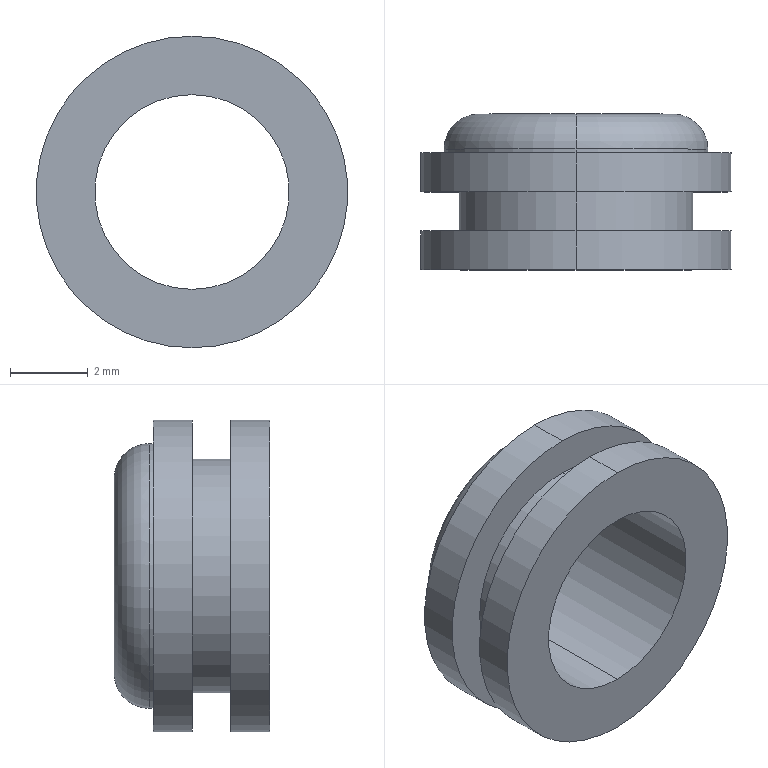Part | SolidWorks | features Revolution 1 | 1 solid | 16 faces | box 8 x 4 x 8 mm | volume 83.088 mm3 | cylinder 10 | plane 4 | torus 2 | commonest cylinder face diameters 8 x4 5 x2 6 x2 6.8 x2
STEP:
#1=CARTESIAN_POINT('',(0.,3.1,-3.4));
#2=VERTEX_POINT('',#1);
#3=CARTESIAN_POINT('',(0.,3.1,3.4));
#4=VERTEX_POINT('',#3);
#5=CARTESIAN_POINT('',(0.,3.1,0.));
#6=DIRECTION('',(0.,-1.,0.));
#7=DIRECTION('',(0.,0.,-1.));
#8=AXIS2_PLACEMENT_3D('',#5,#6,#7);
#9=CIRCLE('',#8,3.4);
#10=EDGE_CURVE('',#2,#4,#9,.T.);
#11=ORIENTED_EDGE('',*,*,#10,.T.);
#12=CARTESIAN_POINT('',(0.,3.,3.4));
#13=VERTEX_POINT('',#12);
#14=CARTESIAN_POINT('',(0.,0.,3.4));
#15=DIRECTION('',(0.,-1.,0.));
#16=VECTOR('',#15,1000.);
#17=LINE('',#14,#16);
#18=EDGE_CURVE('',#4,#13,#17,.T.);
#19=ORIENTED_EDGE('',*,*,#18,.T.);
#20=CARTESIAN_POINT('',(0.,3.,-3.4));
#21=VERTEX_POINT('',#20);
#22=CARTESIAN_POINT('',(0.,3.,0.));
#23=DIRECTION('',(0.,-1.,0.));
#24=DIRECTION('',(0.,0.,-1.));
#25=AXIS2_PLACEMENT_3D('',#22,#23,#24);
#26=CIRCLE('',#25,3.4);
#27=EDGE_CURVE('',#21,#13,#26,.T.);
#28=ORIENTED_EDGE('',*,*,#27,.F.);
#29=CARTESIAN_POINT('',(0.,0.,-3.4));
#30=DIRECTION('',(0.,-1.,0.));
#31=VECTOR('',#30,1000.);
#32=LINE('',#29,#31);
#33=EDGE_CURVE('',#2,#21,#32,.T.);
#34=ORIENTED_EDGE('',*,*,#33,.F.);
#35=EDGE_LOOP('',(#11,#19,#28,#34));
#36=FACE_OUTER_BOUND('',#35,.T.);
#37=CARTESIAN_POINT('',(0.,0.,0.));
#38=DIRECTION('',(0.,-1.,0.));
#39=DIRECTION('',(0.,0.,-1.));
#40=AXIS2_PLACEMENT_3D('',#37,#38,#39);
#41=CYLINDRICAL_SURFACE('',#40,3.4);
#42=ADVANCED_FACE('',(#36),#41,.T.);
#43=CARTESIAN_POINT('',(0.,3.,-4.));
#44=VERTEX_POINT('',#43);
#45=CARTESIAN_POINT('',(0.,3.,4.));
#46=VERTEX_POINT('',#45);
#47=CARTESIAN_POINT('',(0.,3.,0.));
#48=DIRECTION('',(0.,-1.,0.));
#49=DIRECTION('',(0.,0.,-1.));
#50=AXIS2_PLACEMENT_3D('',#47,#48,#49);
#51=CIRCLE('',#50,4.);
#52=EDGE_CURVE('',#44,#46,#51,.T.);
#53=ORIENTED_EDGE('',*,*,#52,.T.);
#54=CARTESIAN_POINT('',(0.,2.,4.));
#55=VERTEX_POINT('',#54);
#56=CARTESIAN_POINT('',(0.,0.,4.));
#57=DIRECTION('',(0.,-1.,0.));
#58=VECTOR('',#57,1000.);
#59=LINE('',#56,#58);
#60=EDGE_CURVE('',#46,#55,#59,.T.);
#61=ORIENTED_EDGE('',*,*,#60,.T.);
#62=CARTESIAN_POINT('',(0.,2.,-4.));
#63=VERTEX_POINT('',#62);
#64=CARTESIAN_POINT('',(0.,2.,0.));
#65=DIRECTION('',(0.,-1.,0.));
#66=DIRECTION('',(0.,0.,-1.));
#67=AXIS2_PLACEMENT_3D('',#64,#65,#66);
#68=CIRCLE('',#67,4.);
#69=EDGE_CURVE('',#63,#55,#68,.T.);
#70=ORIENTED_EDGE('',*,*,#69,.F.);
#71=CARTESIAN_POINT('',(0.,0.,-4.));
#72=DIRECTION('',(0.,-1.,0.));
#73=VECTOR('',#72,1000.);
#74=LINE('',#71,#73);
#75=EDGE_CURVE('',#44,#63,#74,.T.);
#76=ORIENTED_EDGE('',*,*,#75,.F.);
#77=EDGE_LOOP('',(#53,#61,#70,#76));
#78=FACE_OUTER_BOUND('',#77,.T.);
#79=CARTESIAN_POINT('',(0.,0.,0.));
#80=DIRECTION('',(0.,-1.,0.));
#81=DIRECTION('',(0.,0.,-1.));
#82=AXIS2_PLACEMENT_3D('',#79,#80,#81);
#83=CYLINDRICAL_SURFACE('',#82,4.);
#84=ADVANCED_FACE('',(#78),#83,.T.);
#85=CARTESIAN_POINT('',(0.,2.,-3.));
#86=VERTEX_POINT('',#85);
#87=CARTESIAN_POINT('',(0.,2.,3.));
#88=VERTEX_POINT('',#87);
#89=CARTESIAN_POINT('',(0.,2.,0.));
#90=DIRECTION('',(0.,-1.,0.));
#91=DIRECTION('',(0.,0.,-1.));
#92=AXIS2_PLACEMENT_3D('',#89,#90,#91);
#93=CIRCLE('',#92,3.);
#94=EDGE_CURVE('',#86,#88,#93,.T.);
#95=ORIENTED_EDGE('',*,*,#94,.T.);
#96=CARTESIAN_POINT('',(0.,1.,3.));
#97=VERTEX_POINT('',#96);
#98=CARTESIAN_POINT('',(0.,0.,3.));
#99=DIRECTION('',(0.,-1.,0.));
#100=VECTOR('',#99,1000.);
#101=LINE('',#98,#100);
#102=EDGE_CURVE('',#88,#97,#101,.T.);
#103=ORIENTED_EDGE('',*,*,#102,.T.);
#104=CARTESIAN_POINT('',(0.,1.,-3.));
#105=VERTEX_POINT('',#104);
#106=CARTESIAN_POINT('',(0.,1.,0.));
#107=DIRECTION('',(0.,-1.,0.));
#108=DIRECTION('',(0.,0.,-1.));
#109=AXIS2_PLACEMENT_3D('',#106,#107,#108);
#110=CIRCLE('',#109,3.);
#111=EDGE_CURVE('',#105,#97,#110,.T.);
#112=ORIENTED_EDGE('',*,*,#111,.F.);
#113=CARTESIAN_POINT('',(0.,0.,-3.));
#114=DIRECTION('',(0.,-1.,0.));
#115=VECTOR('',#114,1000.);
#116=LINE('',#113,#115);
#117=EDGE_CURVE('',#86,#105,#116,.T.);
#118=ORIENTED_EDGE('',*,*,#117,.F.);
#119=EDGE_LOOP('',(#95,#103,#112,#118));
#120=FACE_OUTER_BOUND('',#119,.T.);
#121=CARTESIAN_POINT('',(0.,0.,0.));
#122=DIRECTION('',(0.,-1.,0.));
#123=DIRECTION('',(0.,0.,-1.));
#124=AXIS2_PLACEMENT_3D('',#121,#122,#123);
#125=CYLINDRICAL_SURFACE('',#124,3.);
#126=ADVANCED_FACE('',(#120),#125,.T.);
#127=CARTESIAN_POINT('',(0.,1.,-4.));
#128=VERTEX_POINT('',#127);
#129=CARTESIAN_POINT('',(0.,1.,4.));
#130=VERTEX_POINT('',#129);
#131=CARTESIAN_POINT('',(0.,1.,0.));
#132=DIRECTION('',(0.,-1.,0.));
#133=DIRECTION('',(0.,0.,-1.));
#134=AXIS2_PLACEMENT_3D('',#131,#132,#133);
#135=CIRCLE('',#134,4.);
#136=EDGE_CURVE('',#128,#130,#135,.T.);
#137=ORIENTED_EDGE('',*,*,#136,.T.);
#138=CARTESIAN_POINT('',(0.,0.,4.));
#139=VERTEX_POINT('',#138);
#140=CARTESIAN_POINT('',(0.,0.,4.));
#141=DIRECTION('',(0.,-1.,0.));
#142=VECTOR('',#141,1000.);
#143=LINE('',#140,#142);
#144=EDGE_CURVE('',#130,#139,#143,.T.);
#145=ORIENTED_EDGE('',*,*,#144,.T.);
#146=CARTESIAN_POINT('',(0.,0.,-4.));
#147=VERTEX_POINT('',#146);
#148=CARTESIAN_POINT('',(0.,0.,0.));
#149=DIRECTION('',(0.,-1.,0.));
#150=DIRECTION('',(0.,0.,-1.));
#151=AXIS2_PLACEMENT_3D('',#148,#149,#150);
#152=CIRCLE('',#151,4.);
#153=EDGE_CURVE('',#147,#139,#152,.T.);
#154=ORIENTED_EDGE('',*,*,#153,.F.);
#155=CARTESIAN_POINT('',(0.,0.,-4.));
#156=DIRECTION('',(0.,-1.,0.));
#157=VECTOR('',#156,1000.);
#158=LINE('',#155,#157);
#159=EDGE_CURVE('',#128,#147,#158,.T.);
#160=ORIENTED_EDGE('',*,*,#159,.F.);
#161=EDGE_LOOP('',(#137,#145,#154,#160));
#162=FACE_OUTER_BOUND('',#161,.T.);
#163=CARTESIAN_POINT('',(0.,0.,0.));
#164=DIRECTION('',(0.,-1.,0.));
#165=DIRECTION('',(0.,0.,-1.));
#166=AXIS2_PLACEMENT_3D('',#163,#164,#165);
#167=CYLINDRICAL_SURFACE('',#166,4.);
#168=ADVANCED_FACE('',(#162),#167,.T.);
#169=CARTESIAN_POINT('',(0.,4.,2.5));
#170=VERTEX_POINT('',#169);
#171=CARTESIAN_POINT('',(0.,4.,-2.5));
#172=VERTEX_POINT('',#171);
#173=CARTESIAN_POINT('',(0.,4.,0.));
#174=DIRECTION('',(0.,-1.,0.));
#175=DIRECTION('',(0.,0.,-1.));
#176=AXIS2_PLACEMENT_3D('',#173,#174,#175);
#177=CIRCLE('',#176,2.5);
#178=EDGE_CURVE('',#170,#172,#177,.T.);
#179=ORIENTED_EDGE('',*,*,#178,.F.);
#180=CARTESIAN_POINT('',(0.,0.,2.5));
#181=VERTEX_POINT('',#180);
#182=CARTESIAN_POINT('',(0.,0.,2.5));
#183=DIRECTION('',(0.,-1.,0.));
#184=VECTOR('',#183,1000.);
#185=LINE('',#182,#184);
#186=EDGE_CURVE('',#170,#181,#185,.T.);
#187=ORIENTED_EDGE('',*,*,#186,.T.);
#188=CARTESIAN_POINT('',(0.,0.,-2.5));
#189=VERTEX_POINT('',#188);
#190=CARTESIAN_POINT('',(0.,0.,0.));
#191=DIRECTION('',(0.,-1.,0.));
#192=DIRECTION('',(0.,0.,-1.));
#193=AXIS2_PLACEMENT_3D('',#190,#191,#192);
#194=CIRCLE('',#193,2.5);
#195=EDGE_CURVE('',#181,#189,#194,.T.);
#196=ORIENTED_EDGE('',*,*,#195,.T.);
#197=CARTESIAN_POINT('',(0.,0.,-2.5));
#198=DIRECTION('',(0.,-1.,0.));
#199=VECTOR('',#198,1000.);
#200=LINE('',#197,#199);
#201=EDGE_CURVE('',#172,#189,#200,.T.);
#202=ORIENTED_EDGE('',*,*,#201,.F.);
#203=EDGE_LOOP('',(#179,#187,#196,#202));
#204=FACE_OUTER_BOUND('',#203,.T.);
#205=CARTESIAN_POINT('',(0.,0.,0.));
#206=DIRECTION('',(0.,-1.,0.));
#207=DIRECTION('',(0.,0.,-1.));
#208=AXIS2_PLACEMENT_3D('',#205,#206,#207);
#209=CYLINDRICAL_SURFACE('',#208,2.5);
#210=ADVANCED_FACE('',(#204),#209,.F.);
#211=CARTESIAN_POINT('',(0.,4.,0.));
#212=DIRECTION('',(0.,-1.,0.));
#213=DIRECTION('',(0.,0.,-1.));
#214=AXIS2_PLACEMENT_3D('',#211,#212,#213);
#215=CIRCLE('',#214,2.5);
#216=EDGE_CURVE('',#172,#170,#215,.T.);
#217=ORIENTED_EDGE('',*,*,#216,.T.);
#218=CARTESIAN_POINT('',(0.,3.1,2.5));
#219=DIRECTION('',(1.,0.,0.));
#220=DIRECTION('',(0.,0.,-1.));
#221=AXIS2_PLACEMENT_3D('',#218,#219,#220);
#222=CIRCLE('',#221,0.9);
#223=EDGE_CURVE('',#170,#4,#222,.T.);
#224=ORIENTED_EDGE('',*,*,#223,.T.);
#225=ORIENTED_EDGE('',*,*,#10,.F.);
#226=CARTESIAN_POINT('',(0.,3.1,-2.5));
#227=DIRECTION('',(-1.,0.,0.));
#228=DIRECTION('',(0.,0.,1.));
#229=AXIS2_PLACEMENT_3D('',#226,#227,#228);
#230=CIRCLE('',#229,0.9);
#231=EDGE_CURVE('',#172,#2,#230,.T.);
#232=ORIENTED_EDGE('',*,*,#231,.F.);
#233=EDGE_LOOP('',(#217,#224,#225,#232));
#234=FACE_OUTER_BOUND('',#233,.T.);
#235=CARTESIAN_POINT('',(0.,3.1,0.));
#236=DIRECTION('',(0.,-1.,0.));
#237=DIRECTION('',(0.,0.,-1.));
#238=AXIS2_PLACEMENT_3D('',#235,#236,#237);
#239=TOROIDAL_SURFACE('',#238,2.5,0.9);
#240=ADVANCED_FACE('',(#234),#239,.T.);
#241=ORIENTED_EDGE('',*,*,#223,.F.);
#242=ORIENTED_EDGE('',*,*,#178,.T.);
#243=ORIENTED_EDGE('',*,*,#231,.T.);
#244=CARTESIAN_POINT('',(0.,3.1,0.));
#245=DIRECTION('',(0.,-1.,0.));
#246=DIRECTION('',(0.,0.,-1.));
#247=AXIS2_PLACEMENT_3D('',#244,#245,#246);
#248=CIRCLE('',#247,3.4);
#249=EDGE_CURVE('',#4,#2,#248,.T.);
#250=ORIENTED_EDGE('',*,*,#249,.F.);
#251=EDGE_LOOP('',(#241,#242,#243,#250));
#252=FACE_OUTER_BOUND('',#251,.T.);
#253=CARTESIAN_POINT('',(0.,3.1,0.));
#254=DIRECTION('',(0.,-1.,0.));
#255=DIRECTION('',(0.,0.,-1.));
#256=AXIS2_PLACEMENT_3D('',#253,#254,#255);
#257=TOROIDAL_SURFACE('',#256,2.5,0.9);
#258=ADVANCED_FACE('',(#252),#257,.T.);
#259=ORIENTED_EDGE('',*,*,#186,.F.);
#260=ORIENTED_EDGE('',*,*,#216,.F.);
#261=ORIENTED_EDGE('',*,*,#201,.T.);
#262=CARTESIAN_POINT('',(0.,0.,0.));
#263=DIRECTION('',(0.,-1.,0.));
#264=DIRECTION('',(0.,0.,-1.));
#265=AXIS2_PLACEMENT_3D('',#262,#263,#264);
#266=CIRCLE('',#265,2.5);
#267=EDGE_CURVE('',#189,#181,#266,.T.);
#268=ORIENTED_EDGE('',*,*,#267,.T.);
#269=EDGE_LOOP('',(#259,#260,#261,#268));
#270=FACE_OUTER_BOUND('',#269,.T.);
#271=CARTESIAN_POINT('',(0.,0.,0.));
#272=DIRECTION('',(0.,-1.,0.));
#273=DIRECTION('',(0.,0.,-1.));
#274=AXIS2_PLACEMENT_3D('',#271,#272,#273);
#275=CYLINDRICAL_SURFACE('',#274,2.5);
#276=ADVANCED_FACE('',(#270),#275,.F.);
#277=ORIENTED_EDGE('',*,*,#153,.T.);
#278=CARTESIAN_POINT('',(0.,0.,0.));
#279=DIRECTION('',(0.,-1.,0.));
#280=DIRECTION('',(0.,0.,-1.));
#281=AXIS2_PLACEMENT_3D('',#278,#279,#280);
#282=CIRCLE('',#281,4.);
#283=EDGE_CURVE('',#139,#147,#282,.T.);
#284=ORIENTED_EDGE('',*,*,#283,.T.);
#285=EDGE_LOOP('',(#277,#284));
#286=FACE_OUTER_BOUND('',#285,.T.);
#287=ORIENTED_EDGE('',*,*,#267,.F.);
#288=ORIENTED_EDGE('',*,*,#195,.F.);
#289=EDGE_LOOP('',(#287,#288));
#290=FACE_BOUND('',#289,.T.);
#291=CARTESIAN_POINT('',(2.5,0.,0.));
#292=DIRECTION('',(0.,-1.,0.));
#293=DIRECTION('',(0.,0.,-1.));
#294=AXIS2_PLACEMENT_3D('',#291,#292,#293);
#295=PLANE('',#294);
#296=ADVANCED_FACE('',(#286,#290),#295,.T.);
#297=ORIENTED_EDGE('',*,*,#144,.F.);
#298=CARTESIAN_POINT('',(0.,1.,0.));
#299=DIRECTION('',(0.,-1.,0.));
#300=DIRECTION('',(0.,0.,-1.));
#301=AXIS2_PLACEMENT_3D('',#298,#299,#300);
#302=CIRCLE('',#301,4.);
#303=EDGE_CURVE('',#130,#128,#302,.T.);
#304=ORIENTED_EDGE('',*,*,#303,.T.);
#305=ORIENTED_EDGE('',*,*,#159,.T.);
#306=ORIENTED_EDGE('',*,*,#283,.F.);
#307=EDGE_LOOP('',(#297,#304,#305,#306));
#308=FACE_OUTER_BOUND('',#307,.T.);
#309=CARTESIAN_POINT('',(0.,0.,0.));
#310=DIRECTION('',(0.,-1.,0.));
#311=DIRECTION('',(0.,0.,-1.));
#312=AXIS2_PLACEMENT_3D('',#309,#310,#311);
#313=CYLINDRICAL_SURFACE('',#312,4.);
#314=ADVANCED_FACE('',(#308),#313,.T.);
#315=ORIENTED_EDGE('',*,*,#111,.T.);
#316=CARTESIAN_POINT('',(0.,1.,0.));
#317=DIRECTION('',(0.,-1.,0.));
#318=DIRECTION('',(0.,0.,-1.));
#319=AXIS2_PLACEMENT_3D('',#316,#317,#318);
#320=CIRCLE('',#319,3.);
#321=EDGE_CURVE('',#97,#105,#320,.T.);
#322=ORIENTED_EDGE('',*,*,#321,.T.);
#323=EDGE_LOOP('',(#315,#322));
#324=FACE_BOUND('',#323,.T.);
#325=ORIENTED_EDGE('',*,*,#136,.F.);
#326=ORIENTED_EDGE('',*,*,#303,.F.);
#327=EDGE_LOOP('',(#325,#326));
#328=FACE_OUTER_BOUND('',#327,.T.);
#329=CARTESIAN_POINT('',(4.,1.,0.));
#330=DIRECTION('',(0.,1.,0.));
#331=DIRECTION('',(0.,0.,1.));
#332=AXIS2_PLACEMENT_3D('',#329,#330,#331);
#333=PLANE('',#332);
#334=ADVANCED_FACE('',(#324,#328),#333,.T.);
#335=ORIENTED_EDGE('',*,*,#102,.F.);
#336=CARTESIAN_POINT('',(0.,2.,0.));
#337=DIRECTION('',(0.,-1.,0.));
#338=DIRECTION('',(0.,0.,-1.));
#339=AXIS2_PLACEMENT_3D('',#336,#337,#338);
#340=CIRCLE('',#339,3.);
#341=EDGE_CURVE('',#88,#86,#340,.T.);
#342=ORIENTED_EDGE('',*,*,#341,.T.);
#343=ORIENTED_EDGE('',*,*,#117,.T.);
#344=ORIENTED_EDGE('',*,*,#321,.F.);
#345=EDGE_LOOP('',(#335,#342,#343,#344));
#346=FACE_OUTER_BOUND('',#345,.T.);
#347=CARTESIAN_POINT('',(0.,0.,0.));
#348=DIRECTION('',(0.,-1.,0.));
#349=DIRECTION('',(0.,0.,-1.));
#350=AXIS2_PLACEMENT_3D('',#347,#348,#349);
#351=CYLINDRICAL_SURFACE('',#350,3.);
#352=ADVANCED_FACE('',(#346),#351,.T.);
#353=ORIENTED_EDGE('',*,*,#69,.T.);
#354=CARTESIAN_POINT('',(0.,2.,0.));
#355=DIRECTION('',(0.,-1.,0.));
#356=DIRECTION('',(0.,0.,-1.));
#357=AXIS2_PLACEMENT_3D('',#354,#355,#356);
#358=CIRCLE('',#357,4.);
#359=EDGE_CURVE('',#55,#63,#358,.T.);
#360=ORIENTED_EDGE('',*,*,#359,.T.);
#361=EDGE_LOOP('',(#353,#360));
#362=FACE_OUTER_BOUND('',#361,.T.);
#363=ORIENTED_EDGE('',*,*,#94,.F.);
#364=ORIENTED_EDGE('',*,*,#341,.F.);
#365=EDGE_LOOP('',(#363,#364));
#366=FACE_BOUND('',#365,.T.);
#367=CARTESIAN_POINT('',(3.,2.,0.));
#368=DIRECTION('',(0.,-1.,0.));
#369=DIRECTION('',(0.,0.,-1.));
#370=AXIS2_PLACEMENT_3D('',#367,#368,#369);
#371=PLANE('',#370);
#372=ADVANCED_FACE('',(#362,#366),#371,.T.);
#373=ORIENTED_EDGE('',*,*,#60,.F.);
#374=CARTESIAN_POINT('',(0.,3.,0.));
#375=DIRECTION('',(0.,-1.,0.));
#376=DIRECTION('',(0.,0.,-1.));
#377=AXIS2_PLACEMENT_3D('',#374,#375,#376);
#378=CIRCLE('',#377,4.);
#379=EDGE_CURVE('',#46,#44,#378,.T.);
#380=ORIENTED_EDGE('',*,*,#379,.T.);
#381=ORIENTED_EDGE('',*,*,#75,.T.);
#382=ORIENTED_EDGE('',*,*,#359,.F.);
#383=EDGE_LOOP('',(#373,#380,#381,#382));
#384=FACE_OUTER_BOUND('',#383,.T.);
#385=CARTESIAN_POINT('',(0.,0.,0.));
#386=DIRECTION('',(0.,-1.,0.));
#387=DIRECTION('',(0.,0.,-1.));
#388=AXIS2_PLACEMENT_3D('',#385,#386,#387);
#389=CYLINDRICAL_SURFACE('',#388,4.);
#390=ADVANCED_FACE('',(#384),#389,.T.);
#391=ORIENTED_EDGE('',*,*,#27,.T.);
#392=CARTESIAN_POINT('',(0.,3.,0.));
#393=DIRECTION('',(0.,-1.,0.));
#394=DIRECTION('',(0.,0.,-1.));
#395=AXIS2_PLACEMENT_3D('',#392,#393,#394);
#396=CIRCLE('',#395,3.4);
#397=EDGE_CURVE('',#13,#21,#396,.T.);
#398=ORIENTED_EDGE('',*,*,#397,.T.);
#399=EDGE_LOOP('',(#391,#398));
#400=FACE_BOUND('',#399,.T.);
#401=ORIENTED_EDGE('',*,*,#52,.F.);
#402=ORIENTED_EDGE('',*,*,#379,.F.);
#403=EDGE_LOOP('',(#401,#402));
#404=FACE_OUTER_BOUND('',#403,.T.);
#405=CARTESIAN_POINT('',(4.,3.,0.));
#406=DIRECTION('',(0.,1.,0.));
#407=DIRECTION('',(0.,0.,1.));
#408=AXIS2_PLACEMENT_3D('',#405,#406,#407);
#409=PLANE('',#408);
#410=ADVANCED_FACE('',(#400,#404),#409,.T.);
#411=ORIENTED_EDGE('',*,*,#18,.F.);
#412=ORIENTED_EDGE('',*,*,#249,.T.);
#413=ORIENTED_EDGE('',*,*,#33,.T.);
#414=ORIENTED_EDGE('',*,*,#397,.F.);
#415=EDGE_LOOP('',(#411,#412,#413,#414));
#416=FACE_OUTER_BOUND('',#415,.T.);
#417=CARTESIAN_POINT('',(0.,0.,0.));
#418=DIRECTION('',(0.,-1.,0.));
#419=DIRECTION('',(0.,0.,-1.));
#420=AXIS2_PLACEMENT_3D('',#417,#418,#419);
#421=CYLINDRICAL_SURFACE('',#420,3.4);
#422=ADVANCED_FACE('',(#416),#421,.T.);
#423=CLOSED_SHELL('',(#42,#84,#126,#168,#210,#240,#258,#276,#296,#314,#334,#352,#372,#390,#410,#422));
#424=MANIFOLD_SOLID_BREP('',#423);
#425=CARTESIAN_POINT('',(0.,0.,0.));
#426=DIRECTION('',(0.,0.,1.));
#427=DIRECTION('',(1.,0.,0.));
#428=AXIS2_PLACEMENT_3D('',#425,#426,#427);
#429=(LENGTH_UNIT()NAMED_UNIT(*)SI_UNIT(.MILLI.,.METRE.));
#430=UNCERTAINTY_MEASURE_WITH_UNIT(LENGTH_MEASURE(0.00001),#429,'','');
#431=(NAMED_UNIT(*)PLANE_ANGLE_UNIT()SI_UNIT($,.RADIAN.));
#432=(NAMED_UNIT(*)SI_UNIT($,.STERADIAN.)SOLID_ANGLE_UNIT());
#433=(GEOMETRIC_REPRESENTATION_CONTEXT(3)GLOBAL_UNCERTAINTY_ASSIGNED_CONTEXT((#430))GLOBAL_UNIT_ASSIGNED_CONTEXT((#429,#431,#432))REPRESENTATION_CONTEXT('',''));
#434=ADVANCED_BREP_SHAPE_REPRESENTATION('',(#424,#428),#433);